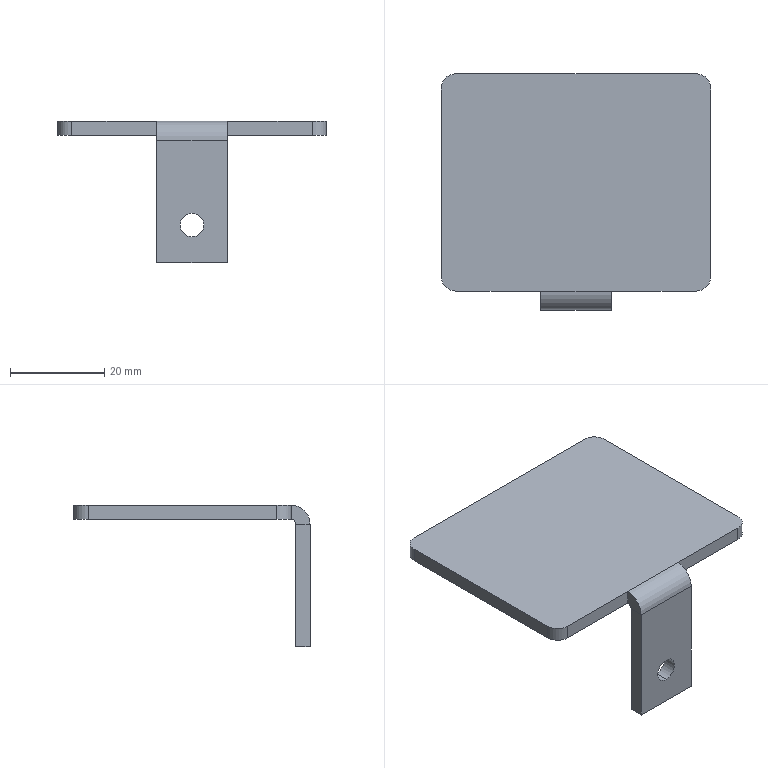Part | SolidWorks | features EdgeFlange 1, Fillet 1, FlatPattern 1, HoleWzd 1, SMBaseFlange 1, SheetMetal 1 | 1 solid | 22 faces | box 57 x 50 x 30 mm | volume 9131 mm3 | plane 14 | cylinder 8 | commonest cylinder face diameters 6 x4 5 x2 2 x1 8 x1
STEP:
#1=CARTESIAN_POINT('',(0.,-24.,-24.5));
#2=VERTEX_POINT('',#1);
#3=CARTESIAN_POINT('',(0.,-24.,-19.5));
#4=VERTEX_POINT('',#3);
#5=CARTESIAN_POINT('',(0.,-24.,-22.));
#6=DIRECTION('',(0.,1.,0.));
#7=DIRECTION('',(0.,0.,1.));
#8=AXIS2_PLACEMENT_3D('',#5,#6,#7);
#9=CIRCLE('',#8,2.5);
#10=EDGE_CURVE('',#2,#4,#9,.T.);
#11=ORIENTED_EDGE('',*,*,#10,.T.);
#12=CARTESIAN_POINT('',(0.,-27.,-19.5));
#13=VERTEX_POINT('',#12);
#14=CARTESIAN_POINT('',(0.,-27.,-19.5));
#15=DIRECTION('',(0.,-1.,0.));
#16=VECTOR('',#15,1000.);
#17=LINE('',#14,#16);
#18=EDGE_CURVE('',#4,#13,#17,.T.);
#19=ORIENTED_EDGE('',*,*,#18,.T.);
#20=CARTESIAN_POINT('',(0.,-27.,-24.5));
#21=VERTEX_POINT('',#20);
#22=CARTESIAN_POINT('',(0.,-27.,-22.));
#23=DIRECTION('',(0.,-1.,0.));
#24=DIRECTION('',(0.,0.,-1.));
#25=AXIS2_PLACEMENT_3D('',#22,#23,#24);
#26=CIRCLE('',#25,2.5);
#27=EDGE_CURVE('',#13,#21,#26,.T.);
#28=ORIENTED_EDGE('',*,*,#27,.T.);
#29=CARTESIAN_POINT('',(0.,-27.,-24.5));
#30=DIRECTION('',(0.,-1.,0.));
#31=VECTOR('',#30,1000.);
#32=LINE('',#29,#31);
#33=EDGE_CURVE('',#2,#21,#32,.T.);
#34=ORIENTED_EDGE('',*,*,#33,.F.);
#35=EDGE_LOOP('',(#11,#19,#28,#34));
#36=FACE_OUTER_BOUND('',#35,.T.);
#37=CARTESIAN_POINT('',(0.,-27.,-22.));
#38=DIRECTION('',(0.,-1.,0.));
#39=DIRECTION('',(0.,0.,-1.));
#40=AXIS2_PLACEMENT_3D('',#37,#38,#39);
#41=CYLINDRICAL_SURFACE('',#40,2.5);
#42=ADVANCED_FACE('',(#36),#41,.F.);
#43=CARTESIAN_POINT('',(-25.5,-23.,0.));
#44=VERTEX_POINT('',#43);
#45=CARTESIAN_POINT('',(-7.5,-23.,0.));
#46=VERTEX_POINT('',#45);
#47=CARTESIAN_POINT('',(-28.5,-23.,0.));
#48=DIRECTION('',(1.,0.,0.));
#49=VECTOR('',#48,1000.);
#50=LINE('',#47,#49);
#51=EDGE_CURVE('',#44,#46,#50,.T.);
#52=ORIENTED_EDGE('',*,*,#51,.F.);
#53=CARTESIAN_POINT('',(-25.5,-23.,-3.));
#54=VERTEX_POINT('',#53);
#55=CARTESIAN_POINT('',(-25.5,-23.,-3.));
#56=DIRECTION('',(0.,0.,-1.));
#57=VECTOR('',#56,1000.);
#58=LINE('',#55,#57);
#59=EDGE_CURVE('',#44,#54,#58,.T.);
#60=ORIENTED_EDGE('',*,*,#59,.T.);
#61=CARTESIAN_POINT('',(-7.5,-23.,-3.));
#62=VERTEX_POINT('',#61);
#63=CARTESIAN_POINT('',(-28.5,-23.,-3.));
#64=DIRECTION('',(1.,0.,0.));
#65=VECTOR('',#64,1000.);
#66=LINE('',#63,#65);
#67=EDGE_CURVE('',#54,#62,#66,.T.);
#68=ORIENTED_EDGE('',*,*,#67,.T.);
#69=CARTESIAN_POINT('',(-7.5,-23.,-3.));
#70=DIRECTION('',(0.,0.,1.));
#71=VECTOR('',#70,1000.);
#72=LINE('',#69,#71);
#73=EDGE_CURVE('',#62,#46,#72,.T.);
#74=ORIENTED_EDGE('',*,*,#73,.T.);
#75=EDGE_LOOP('',(#52,#60,#68,#74));
#76=FACE_OUTER_BOUND('',#75,.T.);
#77=CARTESIAN_POINT('',(-28.5,-23.,-3.));
#78=DIRECTION('',(0.,-1.,0.));
#79=DIRECTION('',(0.,0.,-1.));
#80=AXIS2_PLACEMENT_3D('',#77,#78,#79);
#81=PLANE('',#80);
#82=ADVANCED_FACE('',(#76),#81,.T.);
#83=CARTESIAN_POINT('',(-28.5,20.,-3.));
#84=VERTEX_POINT('',#83);
#85=CARTESIAN_POINT('',(-28.5,-20.,-3.));
#86=VERTEX_POINT('',#85);
#87=CARTESIAN_POINT('',(-28.5,23.,-3.));
#88=DIRECTION('',(0.,-1.,0.));
#89=VECTOR('',#88,1000.);
#90=LINE('',#87,#89);
#91=EDGE_CURVE('',#84,#86,#90,.T.);
#92=ORIENTED_EDGE('',*,*,#91,.T.);
#93=CARTESIAN_POINT('',(-28.5,-20.,0.));
#94=VERTEX_POINT('',#93);
#95=CARTESIAN_POINT('',(-28.5,-20.,-3.));
#96=DIRECTION('',(0.,0.,1.));
#97=VECTOR('',#96,1000.);
#98=LINE('',#95,#97);
#99=EDGE_CURVE('',#86,#94,#98,.T.);
#100=ORIENTED_EDGE('',*,*,#99,.T.);
#101=CARTESIAN_POINT('',(-28.5,20.,0.));
#102=VERTEX_POINT('',#101);
#103=CARTESIAN_POINT('',(-28.5,23.,0.));
#104=DIRECTION('',(0.,-1.,0.));
#105=VECTOR('',#104,1000.);
#106=LINE('',#103,#105);
#107=EDGE_CURVE('',#102,#94,#106,.T.);
#108=ORIENTED_EDGE('',*,*,#107,.F.);
#109=CARTESIAN_POINT('',(-28.5,20.,-3.));
#110=DIRECTION('',(0.,0.,-1.));
#111=VECTOR('',#110,1000.);
#112=LINE('',#109,#111);
#113=EDGE_CURVE('',#102,#84,#112,.T.);
#114=ORIENTED_EDGE('',*,*,#113,.T.);
#115=EDGE_LOOP('',(#92,#100,#108,#114));
#116=FACE_OUTER_BOUND('',#115,.T.);
#117=CARTESIAN_POINT('',(-28.5,23.,-3.));
#118=DIRECTION('',(-1.,0.,0.));
#119=DIRECTION('',(0.,0.,1.));
#120=AXIS2_PLACEMENT_3D('',#117,#118,#119);
#121=PLANE('',#120);
#122=ADVANCED_FACE('',(#116),#121,.T.);
#123=CARTESIAN_POINT('',(25.5,23.,0.));
#124=VERTEX_POINT('',#123);
#125=CARTESIAN_POINT('',(-25.5,23.,0.));
#126=VERTEX_POINT('',#125);
#127=CARTESIAN_POINT('',(-28.5,23.,0.));
#128=DIRECTION('',(-1.,0.,0.));
#129=VECTOR('',#128,1000.);
#130=LINE('',#127,#129);
#131=EDGE_CURVE('',#124,#126,#130,.T.);
#132=ORIENTED_EDGE('',*,*,#131,.F.);
#133=CARTESIAN_POINT('',(25.5,23.,-3.));
#134=VERTEX_POINT('',#133);
#135=CARTESIAN_POINT('',(25.5,23.,-3.));
#136=DIRECTION('',(0.,0.,-1.));
#137=VECTOR('',#136,1000.);
#138=LINE('',#135,#137);
#139=EDGE_CURVE('',#124,#134,#138,.T.);
#140=ORIENTED_EDGE('',*,*,#139,.T.);
#141=CARTESIAN_POINT('',(-25.5,23.,-3.));
#142=VERTEX_POINT('',#141);
#143=CARTESIAN_POINT('',(-28.5,23.,-3.));
#144=DIRECTION('',(-1.,0.,0.));
#145=VECTOR('',#144,1000.);
#146=LINE('',#143,#145);
#147=EDGE_CURVE('',#134,#142,#146,.T.);
#148=ORIENTED_EDGE('',*,*,#147,.T.);
#149=CARTESIAN_POINT('',(-25.5,23.,-3.));
#150=DIRECTION('',(0.,0.,1.));
#151=VECTOR('',#150,1000.);
#152=LINE('',#149,#151);
#153=EDGE_CURVE('',#142,#126,#152,.T.);
#154=ORIENTED_EDGE('',*,*,#153,.T.);
#155=EDGE_LOOP('',(#132,#140,#148,#154));
#156=FACE_OUTER_BOUND('',#155,.T.);
#157=CARTESIAN_POINT('',(-28.5,23.,-3.));
#158=DIRECTION('',(0.,1.,0.));
#159=DIRECTION('',(0.,0.,1.));
#160=AXIS2_PLACEMENT_3D('',#157,#158,#159);
#161=PLANE('',#160);
#162=ADVANCED_FACE('',(#156),#161,.T.);
#163=CARTESIAN_POINT('',(28.5,-20.,0.));
#164=VERTEX_POINT('',#163);
#165=CARTESIAN_POINT('',(28.5,20.,0.));
#166=VERTEX_POINT('',#165);
#167=CARTESIAN_POINT('',(28.5,23.,0.));
#168=DIRECTION('',(0.,1.,0.));
#169=VECTOR('',#168,1000.);
#170=LINE('',#167,#169);
#171=EDGE_CURVE('',#164,#166,#170,.T.);
#172=ORIENTED_EDGE('',*,*,#171,.F.);
#173=CARTESIAN_POINT('',(28.5,-20.,-3.));
#174=VERTEX_POINT('',#173);
#175=CARTESIAN_POINT('',(28.5,-20.,-3.));
#176=DIRECTION('',(0.,0.,-1.));
#177=VECTOR('',#176,1000.);
#178=LINE('',#175,#177);
#179=EDGE_CURVE('',#164,#174,#178,.T.);
#180=ORIENTED_EDGE('',*,*,#179,.T.);
#181=CARTESIAN_POINT('',(28.5,20.,-3.));
#182=VERTEX_POINT('',#181);
#183=CARTESIAN_POINT('',(28.5,23.,-3.));
#184=DIRECTION('',(0.,1.,0.));
#185=VECTOR('',#184,1000.);
#186=LINE('',#183,#185);
#187=EDGE_CURVE('',#174,#182,#186,.T.);
#188=ORIENTED_EDGE('',*,*,#187,.T.);
#189=CARTESIAN_POINT('',(28.5,20.,-3.));
#190=DIRECTION('',(0.,0.,1.));
#191=VECTOR('',#190,1000.);
#192=LINE('',#189,#191);
#193=EDGE_CURVE('',#182,#166,#192,.T.);
#194=ORIENTED_EDGE('',*,*,#193,.T.);
#195=EDGE_LOOP('',(#172,#180,#188,#194));
#196=FACE_OUTER_BOUND('',#195,.T.);
#197=CARTESIAN_POINT('',(28.5,23.,-3.));
#198=DIRECTION('',(1.,0.,0.));
#199=DIRECTION('',(0.,0.,-1.));
#200=AXIS2_PLACEMENT_3D('',#197,#198,#199);
#201=PLANE('',#200);
#202=ADVANCED_FACE('',(#196),#201,.T.);
#203=CARTESIAN_POINT('',(7.5,-23.,-3.));
#204=VERTEX_POINT('',#203);
#205=CARTESIAN_POINT('',(25.5,-23.,-3.));
#206=VERTEX_POINT('',#205);
#207=CARTESIAN_POINT('',(-28.5,-23.,-3.));
#208=DIRECTION('',(1.,0.,0.));
#209=VECTOR('',#208,1000.);
#210=LINE('',#207,#209);
#211=EDGE_CURVE('',#204,#206,#210,.T.);
#212=ORIENTED_EDGE('',*,*,#211,.T.);
#213=CARTESIAN_POINT('',(25.5,-23.,0.));
#214=VERTEX_POINT('',#213);
#215=CARTESIAN_POINT('',(25.5,-23.,-3.));
#216=DIRECTION('',(0.,0.,1.));
#217=VECTOR('',#216,1000.);
#218=LINE('',#215,#217);
#219=EDGE_CURVE('',#206,#214,#218,.T.);
#220=ORIENTED_EDGE('',*,*,#219,.T.);
#221=CARTESIAN_POINT('',(7.5,-23.,0.));
#222=VERTEX_POINT('',#221);
#223=CARTESIAN_POINT('',(-28.5,-23.,0.));
#224=DIRECTION('',(1.,0.,0.));
#225=VECTOR('',#224,1000.);
#226=LINE('',#223,#225);
#227=EDGE_CURVE('',#222,#214,#226,.T.);
#228=ORIENTED_EDGE('',*,*,#227,.F.);
#229=CARTESIAN_POINT('',(7.5,-23.,-3.));
#230=DIRECTION('',(0.,0.,1.));
#231=VECTOR('',#230,1000.);
#232=LINE('',#229,#231);
#233=EDGE_CURVE('',#204,#222,#232,.T.);
#234=ORIENTED_EDGE('',*,*,#233,.F.);
#235=EDGE_LOOP('',(#212,#220,#228,#234));
#236=FACE_OUTER_BOUND('',#235,.T.);
#237=CARTESIAN_POINT('',(-28.5,-23.,-3.));
#238=DIRECTION('',(0.,-1.,0.));
#239=DIRECTION('',(0.,0.,-1.));
#240=AXIS2_PLACEMENT_3D('',#237,#238,#239);
#241=PLANE('',#240);
#242=ADVANCED_FACE('',(#236),#241,.T.);
#243=ORIENTED_EDGE('',*,*,#67,.F.);
#244=CARTESIAN_POINT('',(-25.5,-20.,-3.));
#245=DIRECTION('',(0.,0.,-1.));
#246=DIRECTION('',(1.,0.,0.));
#247=AXIS2_PLACEMENT_3D('',#244,#245,#246);
#248=CIRCLE('',#247,3.);
#249=EDGE_CURVE('',#54,#86,#248,.T.);
#250=ORIENTED_EDGE('',*,*,#249,.T.);
#251=ORIENTED_EDGE('',*,*,#91,.F.);
#252=CARTESIAN_POINT('',(-25.5,20.,-3.));
#253=DIRECTION('',(0.,0.,-1.));
#254=DIRECTION('',(1.,0.,0.));
#255=AXIS2_PLACEMENT_3D('',#252,#253,#254);
#256=CIRCLE('',#255,3.);
#257=EDGE_CURVE('',#84,#142,#256,.T.);
#258=ORIENTED_EDGE('',*,*,#257,.T.);
#259=ORIENTED_EDGE('',*,*,#147,.F.);
#260=CARTESIAN_POINT('',(25.5,20.,-3.));
#261=DIRECTION('',(0.,0.,-1.));
#262=DIRECTION('',(1.,0.,0.));
#263=AXIS2_PLACEMENT_3D('',#260,#261,#262);
#264=CIRCLE('',#263,3.);
#265=EDGE_CURVE('',#134,#182,#264,.T.);
#266=ORIENTED_EDGE('',*,*,#265,.T.);
#267=ORIENTED_EDGE('',*,*,#187,.F.);
#268=CARTESIAN_POINT('',(25.5,-20.,-3.));
#269=DIRECTION('',(0.,0.,-1.));
#270=DIRECTION('',(1.,0.,0.));
#271=AXIS2_PLACEMENT_3D('',#268,#269,#270);
#272=CIRCLE('',#271,3.);
#273=EDGE_CURVE('',#174,#206,#272,.T.);
#274=ORIENTED_EDGE('',*,*,#273,.T.);
#275=ORIENTED_EDGE('',*,*,#211,.F.);
#276=CARTESIAN_POINT('',(-7.5,-23.,-3.));
#277=DIRECTION('',(1.,0.,0.));
#278=VECTOR('',#277,1000.);
#279=LINE('',#276,#278);
#280=EDGE_CURVE('',#62,#204,#279,.T.);
#281=ORIENTED_EDGE('',*,*,#280,.F.);
#282=EDGE_LOOP('',(#243,#250,#251,#258,#259,#266,#267,#274,#275,#281));
#283=FACE_OUTER_BOUND('',#282,.T.);
#284=CARTESIAN_POINT('',(0.,0.,-3.));
#285=DIRECTION('',(0.,0.,1.));
#286=DIRECTION('',(1.,0.,0.));
#287=AXIS2_PLACEMENT_3D('',#284,#285,#286);
#288=PLANE('',#287);
#289=ADVANCED_FACE('',(#283),#288,.F.);
#290=ORIENTED_EDGE('',*,*,#107,.T.);
#291=CARTESIAN_POINT('',(-25.5,-20.,0.));
#292=DIRECTION('',(0.,0.,1.));
#293=DIRECTION('',(1.,0.,0.));
#294=AXIS2_PLACEMENT_3D('',#291,#292,#293);
#295=CIRCLE('',#294,3.);
#296=EDGE_CURVE('',#94,#44,#295,.T.);
#297=ORIENTED_EDGE('',*,*,#296,.T.);
#298=ORIENTED_EDGE('',*,*,#51,.T.);
#299=CARTESIAN_POINT('',(-7.5,-23.,0.));
#300=DIRECTION('',(1.,0.,0.));
#301=VECTOR('',#300,1000.);
#302=LINE('',#299,#301);
#303=EDGE_CURVE('',#46,#222,#302,.T.);
#304=ORIENTED_EDGE('',*,*,#303,.T.);
#305=ORIENTED_EDGE('',*,*,#227,.T.);
#306=CARTESIAN_POINT('',(25.5,-20.,0.));
#307=DIRECTION('',(0.,0.,1.));
#308=DIRECTION('',(1.,0.,0.));
#309=AXIS2_PLACEMENT_3D('',#306,#307,#308);
#310=CIRCLE('',#309,3.);
#311=EDGE_CURVE('',#214,#164,#310,.T.);
#312=ORIENTED_EDGE('',*,*,#311,.T.);
#313=ORIENTED_EDGE('',*,*,#171,.T.);
#314=CARTESIAN_POINT('',(25.5,20.,0.));
#315=DIRECTION('',(0.,0.,1.));
#316=DIRECTION('',(1.,0.,0.));
#317=AXIS2_PLACEMENT_3D('',#314,#315,#316);
#318=CIRCLE('',#317,3.);
#319=EDGE_CURVE('',#166,#124,#318,.T.);
#320=ORIENTED_EDGE('',*,*,#319,.T.);
#321=ORIENTED_EDGE('',*,*,#131,.T.);
#322=CARTESIAN_POINT('',(-25.5,20.,0.));
#323=DIRECTION('',(0.,0.,1.));
#324=DIRECTION('',(1.,0.,0.));
#325=AXIS2_PLACEMENT_3D('',#322,#323,#324);
#326=CIRCLE('',#325,3.);
#327=EDGE_CURVE('',#126,#102,#326,.T.);
#328=ORIENTED_EDGE('',*,*,#327,.T.);
#329=EDGE_LOOP('',(#290,#297,#298,#304,#305,#312,#313,#320,#321,#328));
#330=FACE_OUTER_BOUND('',#329,.T.);
#331=CARTESIAN_POINT('',(0.,0.,0.));
#332=DIRECTION('',(0.,0.,1.));
#333=DIRECTION('',(1.,0.,0.));
#334=AXIS2_PLACEMENT_3D('',#331,#332,#333);
#335=PLANE('',#334);
#336=ADVANCED_FACE('',(#330),#335,.T.);
#337=CARTESIAN_POINT('',(7.5,-24.,-4.));
#338=VERTEX_POINT('',#337);
#339=CARTESIAN_POINT('',(7.5,-27.,-4.));
#340=VERTEX_POINT('',#339);
#341=CARTESIAN_POINT('',(7.5,-27.,-4.));
#342=DIRECTION('',(0.,-1.,0.));
#343=VECTOR('',#342,1000.);
#344=LINE('',#341,#343);
#345=EDGE_CURVE('',#338,#340,#344,.T.);
#346=ORIENTED_EDGE('',*,*,#345,.F.);
#347=CARTESIAN_POINT('',(7.5,-23.,-4.));
#348=DIRECTION('',(1.,0.,0.));
#349=DIRECTION('',(0.,0.,1.));
#350=AXIS2_PLACEMENT_3D('',#347,#348,#349);
#351=CIRCLE('',#350,1.);
#352=EDGE_CURVE('',#204,#338,#351,.T.);
#353=ORIENTED_EDGE('',*,*,#352,.F.);
#354=ORIENTED_EDGE('',*,*,#233,.T.);
#355=CARTESIAN_POINT('',(7.5,-23.,-4.));
#356=DIRECTION('',(1.,0.,0.));
#357=DIRECTION('',(0.,0.,1.));
#358=AXIS2_PLACEMENT_3D('',#355,#356,#357);
#359=CIRCLE('',#358,4.);
#360=EDGE_CURVE('',#222,#340,#359,.T.);
#361=ORIENTED_EDGE('',*,*,#360,.T.);
#362=EDGE_LOOP('',(#346,#353,#354,#361));
#363=FACE_OUTER_BOUND('',#362,.T.);
#364=CARTESIAN_POINT('',(7.5,-23.,-4.));
#365=DIRECTION('',(1.,0.,0.));
#366=DIRECTION('',(0.,0.,-1.));
#367=AXIS2_PLACEMENT_3D('',#364,#365,#366);
#368=PLANE('',#367);
#369=ADVANCED_FACE('',(#363),#368,.T.);
#370=CARTESIAN_POINT('',(-7.5,-24.,-4.));
#371=VERTEX_POINT('',#370);
#372=CARTESIAN_POINT('',(-7.5,-23.,-4.));
#373=DIRECTION('',(-1.,0.,0.));
#374=DIRECTION('',(0.,0.,1.));
#375=AXIS2_PLACEMENT_3D('',#372,#373,#374);
#376=CIRCLE('',#375,1.);
#377=EDGE_CURVE('',#371,#62,#376,.T.);
#378=ORIENTED_EDGE('',*,*,#377,.F.);
#379=CARTESIAN_POINT('',(-7.5,-27.,-4.));
#380=VERTEX_POINT('',#379);
#381=CARTESIAN_POINT('',(-7.5,-24.,-4.));
#382=DIRECTION('',(0.,-1.,0.));
#383=VECTOR('',#382,1000.);
#384=LINE('',#381,#383);
#385=EDGE_CURVE('',#371,#380,#384,.T.);
#386=ORIENTED_EDGE('',*,*,#385,.T.);
#387=CARTESIAN_POINT('',(-7.5,-23.,-4.));
#388=DIRECTION('',(-1.,0.,0.));
#389=DIRECTION('',(0.,0.,1.));
#390=AXIS2_PLACEMENT_3D('',#387,#388,#389);
#391=CIRCLE('',#390,4.);
#392=EDGE_CURVE('',#380,#46,#391,.T.);
#393=ORIENTED_EDGE('',*,*,#392,.T.);
#394=ORIENTED_EDGE('',*,*,#73,.F.);
#395=EDGE_LOOP('',(#378,#386,#393,#394));
#396=FACE_OUTER_BOUND('',#395,.T.);
#397=CARTESIAN_POINT('',(-7.5,-23.,-4.));
#398=DIRECTION('',(1.,0.,0.));
#399=DIRECTION('',(0.,0.,-1.));
#400=AXIS2_PLACEMENT_3D('',#397,#398,#399);
#401=PLANE('',#400);
#402=ADVANCED_FACE('',(#396),#401,.F.);
#403=ORIENTED_EDGE('',*,*,#303,.F.);
#404=ORIENTED_EDGE('',*,*,#392,.F.);
#405=CARTESIAN_POINT('',(7.5,-27.,-4.));
#406=DIRECTION('',(1.,0.,0.));
#407=VECTOR('',#406,1000.);
#408=LINE('',#405,#407);
#409=EDGE_CURVE('',#380,#340,#408,.T.);
#410=ORIENTED_EDGE('',*,*,#409,.T.);
#411=ORIENTED_EDGE('',*,*,#360,.F.);
#412=EDGE_LOOP('',(#403,#404,#410,#411));
#413=FACE_OUTER_BOUND('',#412,.T.);
#414=CARTESIAN_POINT('',(-7.5,-23.,-4.));
#415=DIRECTION('',(-1.,0.,0.));
#416=DIRECTION('',(0.,-1.,0.));
#417=AXIS2_PLACEMENT_3D('',#414,#415,#416);
#418=CYLINDRICAL_SURFACE('',#417,4.);
#419=ADVANCED_FACE('',(#413),#418,.T.);
#420=ORIENTED_EDGE('',*,*,#280,.T.);
#421=ORIENTED_EDGE('',*,*,#352,.T.);
#422=CARTESIAN_POINT('',(7.5,-24.,-4.));
#423=DIRECTION('',(-1.,0.,0.));
#424=VECTOR('',#423,1000.);
#425=LINE('',#422,#424);
#426=EDGE_CURVE('',#338,#371,#425,.T.);
#427=ORIENTED_EDGE('',*,*,#426,.T.);
#428=ORIENTED_EDGE('',*,*,#377,.T.);
#429=EDGE_LOOP('',(#420,#421,#427,#428));
#430=FACE_OUTER_BOUND('',#429,.T.);
#431=CARTESIAN_POINT('',(-7.5,-23.,-4.));
#432=DIRECTION('',(-1.,0.,0.));
#433=DIRECTION('',(0.,-1.,0.));
#434=AXIS2_PLACEMENT_3D('',#431,#432,#433);
#435=CYLINDRICAL_SURFACE('',#434,1.);
#436=ADVANCED_FACE('',(#430),#435,.F.);
#437=ORIENTED_EDGE('',*,*,#385,.F.);
#438=CARTESIAN_POINT('',(-7.5,-24.,-30.));
#439=VERTEX_POINT('',#438);
#440=CARTESIAN_POINT('',(-7.5,-24.,-30.));
#441=DIRECTION('',(0.,0.,-1.));
#442=VECTOR('',#441,1000.);
#443=LINE('',#440,#442);
#444=EDGE_CURVE('',#371,#439,#443,.T.);
#445=ORIENTED_EDGE('',*,*,#444,.T.);
#446=CARTESIAN_POINT('',(-7.5,-27.,-30.));
#447=VERTEX_POINT('',#446);
#448=CARTESIAN_POINT('',(-7.5,-27.,-30.));
#449=DIRECTION('',(0.,1.,0.));
#450=VECTOR('',#449,1000.);
#451=LINE('',#448,#450);
#452=EDGE_CURVE('',#447,#439,#451,.T.);
#453=ORIENTED_EDGE('',*,*,#452,.F.);
#454=CARTESIAN_POINT('',(-7.5,-27.,0.));
#455=DIRECTION('',(0.,0.,-1.));
#456=VECTOR('',#455,1000.);
#457=LINE('',#454,#456);
#458=EDGE_CURVE('',#380,#447,#457,.T.);
#459=ORIENTED_EDGE('',*,*,#458,.F.);
#460=EDGE_LOOP('',(#437,#445,#453,#459));
#461=FACE_OUTER_BOUND('',#460,.T.);
#462=CARTESIAN_POINT('',(-7.5,-27.,-30.));
#463=DIRECTION('',(1.,0.,0.));
#464=DIRECTION('',(0.,0.,-1.));
#465=AXIS2_PLACEMENT_3D('',#462,#463,#464);
#466=PLANE('',#465);
#467=ADVANCED_FACE('',(#461),#466,.F.);
#468=ORIENTED_EDGE('',*,*,#345,.T.);
#469=CARTESIAN_POINT('',(7.5,-27.,-30.));
#470=VERTEX_POINT('',#469);
#471=CARTESIAN_POINT('',(7.5,-27.,0.));
#472=DIRECTION('',(0.,0.,1.));
#473=VECTOR('',#472,1000.);
#474=LINE('',#471,#473);
#475=EDGE_CURVE('',#470,#340,#474,.T.);
#476=ORIENTED_EDGE('',*,*,#475,.F.);
#477=CARTESIAN_POINT('',(7.5,-24.,-30.));
#478=VERTEX_POINT('',#477);
#479=CARTESIAN_POINT('',(7.5,-27.,-30.));
#480=DIRECTION('',(0.,1.,0.));
#481=VECTOR('',#480,1000.);
#482=LINE('',#479,#481);
#483=EDGE_CURVE('',#470,#478,#482,.T.);
#484=ORIENTED_EDGE('',*,*,#483,.T.);
#485=CARTESIAN_POINT('',(7.5,-24.,-3.));
#486=DIRECTION('',(0.,0.,1.));
#487=VECTOR('',#486,1000.);
#488=LINE('',#485,#487);
#489=EDGE_CURVE('',#478,#338,#488,.T.);
#490=ORIENTED_EDGE('',*,*,#489,.T.);
#491=EDGE_LOOP('',(#468,#476,#484,#490));
#492=FACE_OUTER_BOUND('',#491,.T.);
#493=CARTESIAN_POINT('',(7.5,-27.,-3.));
#494=DIRECTION('',(-1.,0.,0.));
#495=DIRECTION('',(0.,0.,1.));
#496=AXIS2_PLACEMENT_3D('',#493,#494,#495);
#497=PLANE('',#496);
#498=ADVANCED_FACE('',(#492),#497,.F.);
#499=CARTESIAN_POINT('',(0.,-27.,-22.));
#500=DIRECTION('',(0.,-1.,0.));
#501=DIRECTION('',(0.,0.,-1.));
#502=AXIS2_PLACEMENT_3D('',#499,#500,#501);
#503=CIRCLE('',#502,2.5);
#504=EDGE_CURVE('',#21,#13,#503,.T.);
#505=ORIENTED_EDGE('',*,*,#504,.F.);
#506=ORIENTED_EDGE('',*,*,#27,.F.);
#507=EDGE_LOOP('',(#505,#506));
#508=FACE_BOUND('',#507,.T.);
#509=ORIENTED_EDGE('',*,*,#409,.F.);
#510=ORIENTED_EDGE('',*,*,#458,.T.);
#511=CARTESIAN_POINT('',(0.,-27.,-30.));
#512=DIRECTION('',(1.,0.,0.));
#513=VECTOR('',#512,1000.);
#514=LINE('',#511,#513);
#515=EDGE_CURVE('',#447,#470,#514,.T.);
#516=ORIENTED_EDGE('',*,*,#515,.T.);
#517=ORIENTED_EDGE('',*,*,#475,.T.);
#518=EDGE_LOOP('',(#509,#510,#516,#517));
#519=FACE_OUTER_BOUND('',#518,.T.);
#520=CARTESIAN_POINT('',(0.,-27.,0.));
#521=DIRECTION('',(0.,1.,0.));
#522=DIRECTION('',(0.,0.,1.));
#523=AXIS2_PLACEMENT_3D('',#520,#521,#522);
#524=PLANE('',#523);
#525=ADVANCED_FACE('',(#508,#519),#524,.F.);
#526=ORIENTED_EDGE('',*,*,#10,.F.);
#527=CARTESIAN_POINT('',(0.,-24.,-22.));
#528=DIRECTION('',(0.,1.,0.));
#529=DIRECTION('',(0.,0.,1.));
#530=AXIS2_PLACEMENT_3D('',#527,#528,#529);
#531=CIRCLE('',#530,2.5);
#532=EDGE_CURVE('',#4,#2,#531,.T.);
#533=ORIENTED_EDGE('',*,*,#532,.F.);
#534=EDGE_LOOP('',(#526,#533));
#535=FACE_BOUND('',#534,.T.);
#536=ORIENTED_EDGE('',*,*,#444,.F.);
#537=ORIENTED_EDGE('',*,*,#426,.F.);
#538=ORIENTED_EDGE('',*,*,#489,.F.);
#539=CARTESIAN_POINT('',(7.5,-24.,-30.));
#540=DIRECTION('',(1.,0.,0.));
#541=VECTOR('',#540,1000.);
#542=LINE('',#539,#541);
#543=EDGE_CURVE('',#439,#478,#542,.T.);
#544=ORIENTED_EDGE('',*,*,#543,.F.);
#545=EDGE_LOOP('',(#536,#537,#538,#544));
#546=FACE_OUTER_BOUND('',#545,.T.);
#547=CARTESIAN_POINT('',(0.,-24.,0.));
#548=DIRECTION('',(0.,1.,0.));
#549=DIRECTION('',(0.,0.,1.));
#550=AXIS2_PLACEMENT_3D('',#547,#548,#549);
#551=PLANE('',#550);
#552=ADVANCED_FACE('',(#535,#546),#551,.T.);
#553=ORIENTED_EDGE('',*,*,#543,.T.);
#554=ORIENTED_EDGE('',*,*,#483,.F.);
#555=ORIENTED_EDGE('',*,*,#515,.F.);
#556=ORIENTED_EDGE('',*,*,#452,.T.);
#557=EDGE_LOOP('',(#553,#554,#555,#556));
#558=FACE_OUTER_BOUND('',#557,.T.);
#559=CARTESIAN_POINT('',(7.5,-27.,-30.));
#560=DIRECTION('',(0.,0.,1.));
#561=DIRECTION('',(0.,-1.,0.));
#562=AXIS2_PLACEMENT_3D('',#559,#560,#561);
#563=PLANE('',#562);
#564=ADVANCED_FACE('',(#558),#563,.F.);
#565=ORIENTED_EDGE('',*,*,#18,.F.);
#566=ORIENTED_EDGE('',*,*,#532,.T.);
#567=ORIENTED_EDGE('',*,*,#33,.T.);
#568=ORIENTED_EDGE('',*,*,#504,.T.);
#569=EDGE_LOOP('',(#565,#566,#567,#568));
#570=FACE_OUTER_BOUND('',#569,.T.);
#571=CARTESIAN_POINT('',(0.,-27.,-22.));
#572=DIRECTION('',(0.,-1.,0.));
#573=DIRECTION('',(0.,0.,-1.));
#574=AXIS2_PLACEMENT_3D('',#571,#572,#573);
#575=CYLINDRICAL_SURFACE('',#574,2.5);
#576=ADVANCED_FACE('',(#570),#575,.F.);
#577=ORIENTED_EDGE('',*,*,#249,.F.);
#578=ORIENTED_EDGE('',*,*,#59,.F.);
#579=ORIENTED_EDGE('',*,*,#296,.F.);
#580=ORIENTED_EDGE('',*,*,#99,.F.);
#581=EDGE_LOOP('',(#577,#578,#579,#580));
#582=FACE_OUTER_BOUND('',#581,.T.);
#583=CARTESIAN_POINT('',(-25.5,-20.,-3.));
#584=DIRECTION('',(0.,0.,1.));
#585=DIRECTION('',(1.,0.,0.));
#586=AXIS2_PLACEMENT_3D('',#583,#584,#585);
#587=CYLINDRICAL_SURFACE('',#586,3.);
#588=ADVANCED_FACE('',(#582),#587,.T.);
#589=ORIENTED_EDGE('',*,*,#273,.F.);
#590=ORIENTED_EDGE('',*,*,#179,.F.);
#591=ORIENTED_EDGE('',*,*,#311,.F.);
#592=ORIENTED_EDGE('',*,*,#219,.F.);
#593=EDGE_LOOP('',(#589,#590,#591,#592));
#594=FACE_OUTER_BOUND('',#593,.T.);
#595=CARTESIAN_POINT('',(25.5,-20.,-3.));
#596=DIRECTION('',(0.,0.,1.));
#597=DIRECTION('',(1.,0.,0.));
#598=AXIS2_PLACEMENT_3D('',#595,#596,#597);
#599=CYLINDRICAL_SURFACE('',#598,3.);
#600=ADVANCED_FACE('',(#594),#599,.T.);
#601=ORIENTED_EDGE('',*,*,#265,.F.);
#602=ORIENTED_EDGE('',*,*,#139,.F.);
#603=ORIENTED_EDGE('',*,*,#319,.F.);
#604=ORIENTED_EDGE('',*,*,#193,.F.);
#605=EDGE_LOOP('',(#601,#602,#603,#604));
#606=FACE_OUTER_BOUND('',#605,.T.);
#607=CARTESIAN_POINT('',(25.5,20.,-3.));
#608=DIRECTION('',(0.,0.,1.));
#609=DIRECTION('',(1.,0.,0.));
#610=AXIS2_PLACEMENT_3D('',#607,#608,#609);
#611=CYLINDRICAL_SURFACE('',#610,3.);
#612=ADVANCED_FACE('',(#606),#611,.T.);
#613=ORIENTED_EDGE('',*,*,#257,.F.);
#614=ORIENTED_EDGE('',*,*,#113,.F.);
#615=ORIENTED_EDGE('',*,*,#327,.F.);
#616=ORIENTED_EDGE('',*,*,#153,.F.);
#617=EDGE_LOOP('',(#613,#614,#615,#616));
#618=FACE_OUTER_BOUND('',#617,.T.);
#619=CARTESIAN_POINT('',(-25.5,20.,-3.));
#620=DIRECTION('',(0.,0.,1.));
#621=DIRECTION('',(1.,0.,0.));
#622=AXIS2_PLACEMENT_3D('',#619,#620,#621);
#623=CYLINDRICAL_SURFACE('',#622,3.);
#624=ADVANCED_FACE('',(#618),#623,.T.);
#625=CLOSED_SHELL('',(#42,#82,#122,#162,#202,#242,#289,#336,#369,#402,#419,#436,#467,#498,#525,#552,#564,#576,#588,#600,#612,#624));
#626=MANIFOLD_SOLID_BREP('',#625);
#627=CARTESIAN_POINT('',(0.,0.,0.));
#628=DIRECTION('',(0.,0.,1.));
#629=DIRECTION('',(1.,0.,0.));
#630=AXIS2_PLACEMENT_3D('',#627,#628,#629);
#631=(LENGTH_UNIT()NAMED_UNIT(*)SI_UNIT(.MILLI.,.METRE.));
#632=UNCERTAINTY_MEASURE_WITH_UNIT(LENGTH_MEASURE(0.00001),#631,'','');
#633=(NAMED_UNIT(*)PLANE_ANGLE_UNIT()SI_UNIT($,.RADIAN.));
#634=(NAMED_UNIT(*)SI_UNIT($,.STERADIAN.)SOLID_ANGLE_UNIT());
#635=(GEOMETRIC_REPRESENTATION_CONTEXT(3)GLOBAL_UNCERTAINTY_ASSIGNED_CONTEXT((#632))GLOBAL_UNIT_ASSIGNED_CONTEXT((#631,#633,#634))REPRESENTATION_CONTEXT('',''));
#636=ADVANCED_BREP_SHAPE_REPRESENTATION('',(#626,#630),#635);